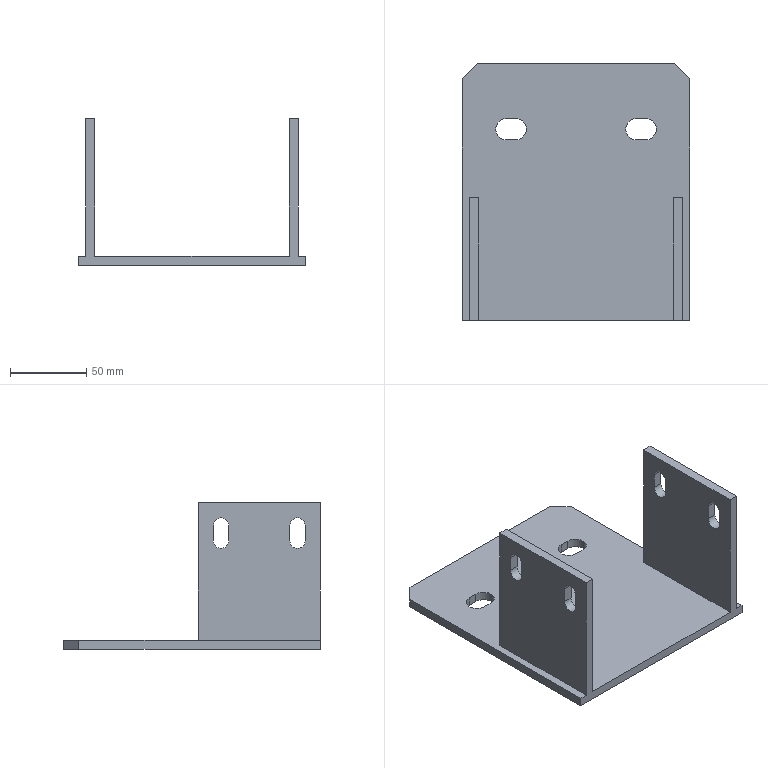Part | STEP file | Guide shoe upper bracket | 1 solid | 42 faces | box 149 x 168 x 96 mm | volume 228852 mm3 | plane 28 | cylinder 14 | commonest cylinder face diameters 10 x8 14 x6